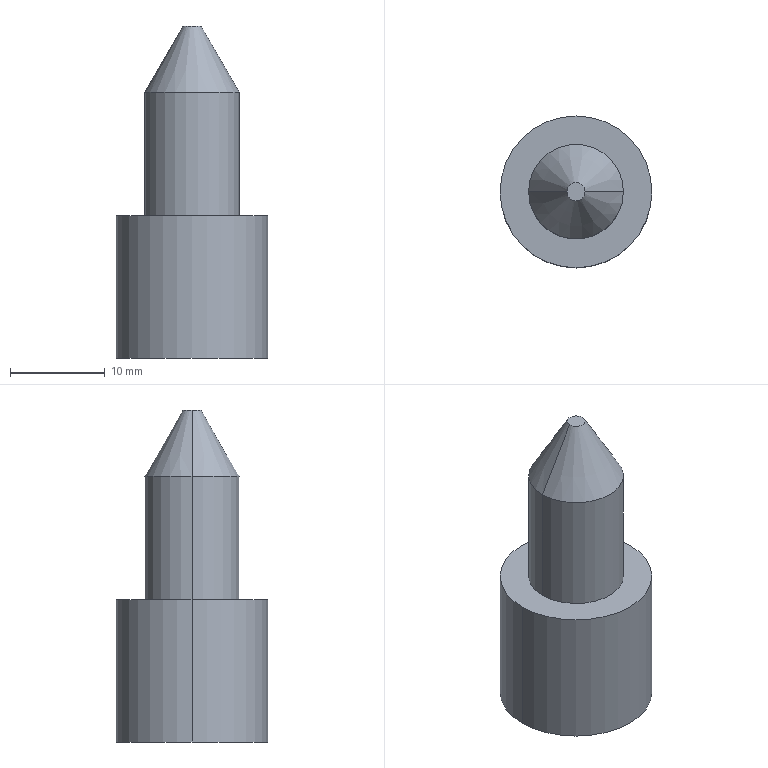Part | SolidWorks | features BaseBody 1 | 1 solid | 13 faces | box 16 x 16 x 35 mm | volume 4084 mm3 | cylinder 6 | cone 4 | plane 3 | commonest cylinder face diameters 4.2 x2 10 x2 16 x2
STEP:
#1=CARTESIAN_POINT('',(2.1,0.,12.4));
#2=VERTEX_POINT('',#1);
#3=CARTESIAN_POINT('',(2.1,0.,0.));
#4=VERTEX_POINT('',#3);
#5=CARTESIAN_POINT('',(2.1,0.,0.));
#6=DIRECTION('',(0.,0.,-1.));
#7=VECTOR('',#6,1000.);
#8=LINE('',#5,#7);
#9=EDGE_CURVE('',#2,#4,#8,.T.);
#10=ORIENTED_EDGE('',*,*,#9,.F.);
#11=CARTESIAN_POINT('',(-2.1,0.,12.4));
#12=VERTEX_POINT('',#11);
#13=CARTESIAN_POINT('',(0.,0.,12.4));
#14=DIRECTION('',(0.,0.,-1.));
#15=DIRECTION('',(-1.,0.,0.));
#16=AXIS2_PLACEMENT_3D('',#13,#14,#15);
#17=CIRCLE('',#16,2.1);
#18=EDGE_CURVE('',#12,#2,#17,.T.);
#19=ORIENTED_EDGE('',*,*,#18,.F.);
#20=CARTESIAN_POINT('',(-2.1,0.,0.));
#21=VERTEX_POINT('',#20);
#22=CARTESIAN_POINT('',(-2.1,0.,0.));
#23=DIRECTION('',(0.,0.,-1.));
#24=VECTOR('',#23,1000.);
#25=LINE('',#22,#24);
#26=EDGE_CURVE('',#12,#21,#25,.T.);
#27=ORIENTED_EDGE('',*,*,#26,.T.);
#28=CARTESIAN_POINT('',(0.,0.,0.));
#29=DIRECTION('',(0.,0.,-1.));
#30=DIRECTION('',(-1.,0.,0.));
#31=AXIS2_PLACEMENT_3D('',#28,#29,#30);
#32=CIRCLE('',#31,2.1);
#33=EDGE_CURVE('',#21,#4,#32,.T.);
#34=ORIENTED_EDGE('',*,*,#33,.T.);
#35=EDGE_LOOP('',(#10,#19,#27,#34));
#36=FACE_OUTER_BOUND('',#35,.T.);
#37=CARTESIAN_POINT('',(0.,0.,0.));
#38=DIRECTION('',(0.,0.,-1.));
#39=DIRECTION('',(-1.,0.,0.));
#40=AXIS2_PLACEMENT_3D('',#37,#38,#39);
#41=CYLINDRICAL_SURFACE('',#40,2.1);
#42=ADVANCED_FACE('',(#36),#41,.F.);
#43=CARTESIAN_POINT('',(0.,0.,13.662));
#44=VERTEX_POINT('',#43);
#45=CARTESIAN_POINT('',(2.1,0.,12.4));
#46=DIRECTION('',(0.8572,0.,-0.515));
#47=VECTOR('',#46,1000.);
#48=LINE('',#45,#47);
#49=EDGE_CURVE('',#44,#2,#48,.T.);
#50=ORIENTED_EDGE('',*,*,#49,.F.);
#51=CARTESIAN_POINT('',(-2.1,0.,12.4));
#52=DIRECTION('',(-0.8572,0.,-0.515));
#53=VECTOR('',#52,1000.);
#54=LINE('',#51,#53);
#55=EDGE_CURVE('',#44,#12,#54,.T.);
#56=ORIENTED_EDGE('',*,*,#55,.T.);
#57=ORIENTED_EDGE('',*,*,#18,.T.);
#58=EDGE_LOOP('',(#50,#56,#57));
#59=FACE_OUTER_BOUND('',#58,.T.);
#60=CARTESIAN_POINT('',(0.,0.,12.4));
#61=DIRECTION('',(0.,0.,-1.));
#62=DIRECTION('',(-1.,0.,0.));
#63=AXIS2_PLACEMENT_3D('',#60,#61,#62);
#64=CONICAL_SURFACE('',#63,2.1,1.03);
#65=ADVANCED_FACE('',(#59),#64,.F.);
#66=CARTESIAN_POINT('',(0.9585,0.,35.));
#67=VERTEX_POINT('',#66);
#68=CARTESIAN_POINT('',(5.,0.,28.));
#69=VERTEX_POINT('',#68);
#70=CARTESIAN_POINT('',(0.9585,0.,35.));
#71=DIRECTION('',(0.5,0.,-0.866));
#72=VECTOR('',#71,1000.);
#73=LINE('',#70,#72);
#74=EDGE_CURVE('',#67,#69,#73,.T.);
#75=ORIENTED_EDGE('',*,*,#74,.F.);
#76=CARTESIAN_POINT('',(-0.9585,0.,35.));
#77=VERTEX_POINT('',#76);
#78=CARTESIAN_POINT('',(0.,0.,35.));
#79=DIRECTION('',(0.,0.,1.));
#80=DIRECTION('',(1.,0.,0.));
#81=AXIS2_PLACEMENT_3D('',#78,#79,#80);
#82=CIRCLE('',#81,0.9585);
#83=EDGE_CURVE('',#77,#67,#82,.T.);
#84=ORIENTED_EDGE('',*,*,#83,.F.);
#85=CARTESIAN_POINT('',(-5.,0.,28.));
#86=VERTEX_POINT('',#85);
#87=CARTESIAN_POINT('',(-0.9585,0.,35.));
#88=DIRECTION('',(-0.5,0.,-0.866));
#89=VECTOR('',#88,1000.);
#90=LINE('',#87,#89);
#91=EDGE_CURVE('',#77,#86,#90,.T.);
#92=ORIENTED_EDGE('',*,*,#91,.T.);
#93=CARTESIAN_POINT('',(0.,0.,28.));
#94=DIRECTION('',(0.,0.,-1.));
#95=DIRECTION('',(1.,0.,0.));
#96=AXIS2_PLACEMENT_3D('',#93,#94,#95);
#97=CIRCLE('',#96,5.);
#98=EDGE_CURVE('',#69,#86,#97,.T.);
#99=ORIENTED_EDGE('',*,*,#98,.F.);
#100=EDGE_LOOP('',(#75,#84,#92,#99));
#101=FACE_OUTER_BOUND('',#100,.T.);
#102=CARTESIAN_POINT('',(0.,0.,35.));
#103=DIRECTION('',(0.,0.,-1.));
#104=DIRECTION('',(-1.,0.,0.));
#105=AXIS2_PLACEMENT_3D('',#102,#103,#104);
#106=CONICAL_SURFACE('',#105,0.9585,0.5236);
#107=ADVANCED_FACE('',(#101),#106,.T.);
#108=ORIENTED_EDGE('',*,*,#83,.T.);
#109=CARTESIAN_POINT('',(0.,0.,35.));
#110=DIRECTION('',(0.,0.,1.));
#111=DIRECTION('',(1.,0.,0.));
#112=AXIS2_PLACEMENT_3D('',#109,#110,#111);
#113=CIRCLE('',#112,0.9585);
#114=EDGE_CURVE('',#67,#77,#113,.T.);
#115=ORIENTED_EDGE('',*,*,#114,.T.);
#116=EDGE_LOOP('',(#108,#115));
#117=FACE_OUTER_BOUND('',#116,.T.);
#118=CARTESIAN_POINT('',(0.,0.,35.));
#119=DIRECTION('',(0.,0.,1.));
#120=DIRECTION('',(1.,0.,0.));
#121=AXIS2_PLACEMENT_3D('',#118,#119,#120);
#122=PLANE('',#121);
#123=ADVANCED_FACE('',(#117),#122,.T.);
#124=CARTESIAN_POINT('',(5.,0.,15.));
#125=VERTEX_POINT('',#124);
#126=CARTESIAN_POINT('',(5.,0.,35.));
#127=DIRECTION('',(0.,0.,-1.));
#128=VECTOR('',#127,1000.);
#129=LINE('',#126,#128);
#130=EDGE_CURVE('',#69,#125,#129,.T.);
#131=ORIENTED_EDGE('',*,*,#130,.F.);
#132=ORIENTED_EDGE('',*,*,#98,.T.);
#133=CARTESIAN_POINT('',(-5.,0.,15.));
#134=VERTEX_POINT('',#133);
#135=CARTESIAN_POINT('',(-5.,0.,35.));
#136=DIRECTION('',(0.,0.,-1.));
#137=VECTOR('',#136,1000.);
#138=LINE('',#135,#137);
#139=EDGE_CURVE('',#86,#134,#138,.T.);
#140=ORIENTED_EDGE('',*,*,#139,.T.);
#141=CARTESIAN_POINT('',(0.,0.,15.));
#142=DIRECTION('',(0.,0.,1.));
#143=DIRECTION('',(1.,0.,0.));
#144=AXIS2_PLACEMENT_3D('',#141,#142,#143);
#145=CIRCLE('',#144,5.);
#146=EDGE_CURVE('',#134,#125,#145,.T.);
#147=ORIENTED_EDGE('',*,*,#146,.T.);
#148=EDGE_LOOP('',(#131,#132,#140,#147));
#149=FACE_OUTER_BOUND('',#148,.T.);
#150=CARTESIAN_POINT('',(0.,0.,35.));
#151=DIRECTION('',(0.,0.,-1.));
#152=DIRECTION('',(-1.,0.,0.));
#153=AXIS2_PLACEMENT_3D('',#150,#151,#152);
#154=CYLINDRICAL_SURFACE('',#153,5.);
#155=ADVANCED_FACE('',(#149),#154,.T.);
#156=ORIENTED_EDGE('',*,*,#33,.F.);
#157=CARTESIAN_POINT('',(0.,0.,0.));
#158=DIRECTION('',(0.,0.,-1.));
#159=DIRECTION('',(-1.,0.,0.));
#160=AXIS2_PLACEMENT_3D('',#157,#158,#159);
#161=CIRCLE('',#160,2.1);
#162=EDGE_CURVE('',#4,#21,#161,.T.);
#163=ORIENTED_EDGE('',*,*,#162,.F.);
#164=EDGE_LOOP('',(#156,#163));
#165=FACE_BOUND('',#164,.T.);
#166=CARTESIAN_POINT('',(-8.,0.,0.));
#167=VERTEX_POINT('',#166);
#168=CARTESIAN_POINT('',(8.,0.,0.));
#169=VERTEX_POINT('',#168);
#170=CARTESIAN_POINT('',(0.,0.,0.));
#171=DIRECTION('',(0.,0.,1.));
#172=DIRECTION('',(1.,0.,0.));
#173=AXIS2_PLACEMENT_3D('',#170,#171,#172);
#174=CIRCLE('',#173,8.);
#175=EDGE_CURVE('',#167,#169,#174,.T.);
#176=ORIENTED_EDGE('',*,*,#175,.F.);
#177=CARTESIAN_POINT('',(0.,0.,0.));
#178=DIRECTION('',(0.,0.,1.));
#179=DIRECTION('',(1.,0.,0.));
#180=AXIS2_PLACEMENT_3D('',#177,#178,#179);
#181=CIRCLE('',#180,8.);
#182=EDGE_CURVE('',#169,#167,#181,.T.);
#183=ORIENTED_EDGE('',*,*,#182,.F.);
#184=EDGE_LOOP('',(#176,#183));
#185=FACE_OUTER_BOUND('',#184,.T.);
#186=CARTESIAN_POINT('',(0.,0.,0.));
#187=DIRECTION('',(0.,0.,1.));
#188=DIRECTION('',(1.,0.,0.));
#189=AXIS2_PLACEMENT_3D('',#186,#187,#188);
#190=PLANE('',#189);
#191=ADVANCED_FACE('',(#165,#185),#190,.F.);
#192=ORIENTED_EDGE('',*,*,#146,.F.);
#193=CARTESIAN_POINT('',(0.,0.,15.));
#194=DIRECTION('',(0.,0.,1.));
#195=DIRECTION('',(1.,0.,0.));
#196=AXIS2_PLACEMENT_3D('',#193,#194,#195);
#197=CIRCLE('',#196,5.);
#198=EDGE_CURVE('',#125,#134,#197,.T.);
#199=ORIENTED_EDGE('',*,*,#198,.F.);
#200=EDGE_LOOP('',(#192,#199));
#201=FACE_BOUND('',#200,.T.);
#202=CARTESIAN_POINT('',(-8.,0.,15.));
#203=VERTEX_POINT('',#202);
#204=CARTESIAN_POINT('',(8.,0.,15.));
#205=VERTEX_POINT('',#204);
#206=CARTESIAN_POINT('',(0.,0.,15.));
#207=DIRECTION('',(0.,0.,1.));
#208=DIRECTION('',(1.,0.,0.));
#209=AXIS2_PLACEMENT_3D('',#206,#207,#208);
#210=CIRCLE('',#209,8.);
#211=EDGE_CURVE('',#203,#205,#210,.T.);
#212=ORIENTED_EDGE('',*,*,#211,.T.);
#213=CARTESIAN_POINT('',(0.,0.,15.));
#214=DIRECTION('',(0.,0.,1.));
#215=DIRECTION('',(1.,0.,0.));
#216=AXIS2_PLACEMENT_3D('',#213,#214,#215);
#217=CIRCLE('',#216,8.);
#218=EDGE_CURVE('',#205,#203,#217,.T.);
#219=ORIENTED_EDGE('',*,*,#218,.T.);
#220=EDGE_LOOP('',(#212,#219));
#221=FACE_OUTER_BOUND('',#220,.T.);
#222=CARTESIAN_POINT('',(0.,0.,15.));
#223=DIRECTION('',(0.,0.,1.));
#224=DIRECTION('',(1.,0.,0.));
#225=AXIS2_PLACEMENT_3D('',#222,#223,#224);
#226=PLANE('',#225);
#227=ADVANCED_FACE('',(#201,#221),#226,.T.);
#228=CARTESIAN_POINT('',(8.,0.,15.));
#229=DIRECTION('',(0.,0.,-1.));
#230=VECTOR('',#229,1000.);
#231=LINE('',#228,#230);
#232=EDGE_CURVE('',#205,#169,#231,.T.);
#233=ORIENTED_EDGE('',*,*,#232,.F.);
#234=ORIENTED_EDGE('',*,*,#211,.F.);
#235=CARTESIAN_POINT('',(-8.,0.,15.));
#236=DIRECTION('',(0.,0.,-1.));
#237=VECTOR('',#236,1000.);
#238=LINE('',#235,#237);
#239=EDGE_CURVE('',#203,#167,#238,.T.);
#240=ORIENTED_EDGE('',*,*,#239,.T.);
#241=ORIENTED_EDGE('',*,*,#175,.T.);
#242=EDGE_LOOP('',(#233,#234,#240,#241));
#243=FACE_OUTER_BOUND('',#242,.T.);
#244=CARTESIAN_POINT('',(0.,0.,15.));
#245=DIRECTION('',(0.,0.,-1.));
#246=DIRECTION('',(-1.,0.,0.));
#247=AXIS2_PLACEMENT_3D('',#244,#245,#246);
#248=CYLINDRICAL_SURFACE('',#247,8.);
#249=ADVANCED_FACE('',(#243),#248,.T.);
#250=ORIENTED_EDGE('',*,*,#218,.F.);
#251=ORIENTED_EDGE('',*,*,#232,.T.);
#252=ORIENTED_EDGE('',*,*,#182,.T.);
#253=ORIENTED_EDGE('',*,*,#239,.F.);
#254=EDGE_LOOP('',(#250,#251,#252,#253));
#255=FACE_OUTER_BOUND('',#254,.T.);
#256=CARTESIAN_POINT('',(0.,0.,15.));
#257=DIRECTION('',(0.,0.,-1.));
#258=DIRECTION('',(-1.,0.,0.));
#259=AXIS2_PLACEMENT_3D('',#256,#257,#258);
#260=CYLINDRICAL_SURFACE('',#259,8.);
#261=ADVANCED_FACE('',(#255),#260,.T.);
#262=CARTESIAN_POINT('',(0.,0.,28.));
#263=DIRECTION('',(0.,0.,-1.));
#264=DIRECTION('',(1.,0.,0.));
#265=AXIS2_PLACEMENT_3D('',#262,#263,#264);
#266=CIRCLE('',#265,5.);
#267=EDGE_CURVE('',#86,#69,#266,.T.);
#268=ORIENTED_EDGE('',*,*,#267,.T.);
#269=ORIENTED_EDGE('',*,*,#130,.T.);
#270=ORIENTED_EDGE('',*,*,#198,.T.);
#271=ORIENTED_EDGE('',*,*,#139,.F.);
#272=EDGE_LOOP('',(#268,#269,#270,#271));
#273=FACE_OUTER_BOUND('',#272,.T.);
#274=CARTESIAN_POINT('',(0.,0.,35.));
#275=DIRECTION('',(0.,0.,-1.));
#276=DIRECTION('',(-1.,0.,0.));
#277=AXIS2_PLACEMENT_3D('',#274,#275,#276);
#278=CYLINDRICAL_SURFACE('',#277,5.);
#279=ADVANCED_FACE('',(#273),#278,.T.);
#280=ORIENTED_EDGE('',*,*,#114,.F.);
#281=ORIENTED_EDGE('',*,*,#74,.T.);
#282=ORIENTED_EDGE('',*,*,#267,.F.);
#283=ORIENTED_EDGE('',*,*,#91,.F.);
#284=EDGE_LOOP('',(#280,#281,#282,#283));
#285=FACE_OUTER_BOUND('',#284,.T.);
#286=CARTESIAN_POINT('',(0.,0.,35.));
#287=DIRECTION('',(0.,0.,-1.));
#288=DIRECTION('',(-1.,0.,0.));
#289=AXIS2_PLACEMENT_3D('',#286,#287,#288);
#290=CONICAL_SURFACE('',#289,0.9585,0.5236);
#291=ADVANCED_FACE('',(#285),#290,.T.);
#292=ORIENTED_EDGE('',*,*,#55,.F.);
#293=ORIENTED_EDGE('',*,*,#49,.T.);
#294=CARTESIAN_POINT('',(0.,0.,12.4));
#295=DIRECTION('',(0.,0.,-1.));
#296=DIRECTION('',(-1.,0.,0.));
#297=AXIS2_PLACEMENT_3D('',#294,#295,#296);
#298=CIRCLE('',#297,2.1);
#299=EDGE_CURVE('',#2,#12,#298,.T.);
#300=ORIENTED_EDGE('',*,*,#299,.T.);
#301=EDGE_LOOP('',(#292,#293,#300));
#302=FACE_OUTER_BOUND('',#301,.T.);
#303=CARTESIAN_POINT('',(0.,0.,12.4));
#304=DIRECTION('',(0.,0.,-1.));
#305=DIRECTION('',(-1.,0.,0.));
#306=AXIS2_PLACEMENT_3D('',#303,#304,#305);
#307=CONICAL_SURFACE('',#306,2.1,1.03);
#308=ADVANCED_FACE('',(#302),#307,.F.);
#309=ORIENTED_EDGE('',*,*,#299,.F.);
#310=ORIENTED_EDGE('',*,*,#9,.T.);
#311=ORIENTED_EDGE('',*,*,#162,.T.);
#312=ORIENTED_EDGE('',*,*,#26,.F.);
#313=EDGE_LOOP('',(#309,#310,#311,#312));
#314=FACE_OUTER_BOUND('',#313,.T.);
#315=CARTESIAN_POINT('',(0.,0.,0.));
#316=DIRECTION('',(0.,0.,-1.));
#317=DIRECTION('',(-1.,0.,0.));
#318=AXIS2_PLACEMENT_3D('',#315,#316,#317);
#319=CYLINDRICAL_SURFACE('',#318,2.1);
#320=ADVANCED_FACE('',(#314),#319,.F.);
#321=CLOSED_SHELL('',(#42,#65,#107,#123,#155,#191,#227,#249,#261,#279,#291,#308,#320));
#322=MANIFOLD_SOLID_BREP('',#321);
#323=CARTESIAN_POINT('',(0.,0.,0.));
#324=DIRECTION('',(0.,0.,1.));
#325=DIRECTION('',(1.,0.,0.));
#326=AXIS2_PLACEMENT_3D('',#323,#324,#325);
#327=(LENGTH_UNIT()NAMED_UNIT(*)SI_UNIT(.MILLI.,.METRE.));
#328=UNCERTAINTY_MEASURE_WITH_UNIT(LENGTH_MEASURE(0.00001),#327,'','');
#329=(NAMED_UNIT(*)PLANE_ANGLE_UNIT()SI_UNIT($,.RADIAN.));
#330=(NAMED_UNIT(*)SI_UNIT($,.STERADIAN.)SOLID_ANGLE_UNIT());
#331=(GEOMETRIC_REPRESENTATION_CONTEXT(3)GLOBAL_UNCERTAINTY_ASSIGNED_CONTEXT((#328))GLOBAL_UNIT_ASSIGNED_CONTEXT((#327,#329,#330))REPRESENTATION_CONTEXT('',''));
#332=ADVANCED_BREP_SHAPE_REPRESENTATION('',(#322,#326),#331);